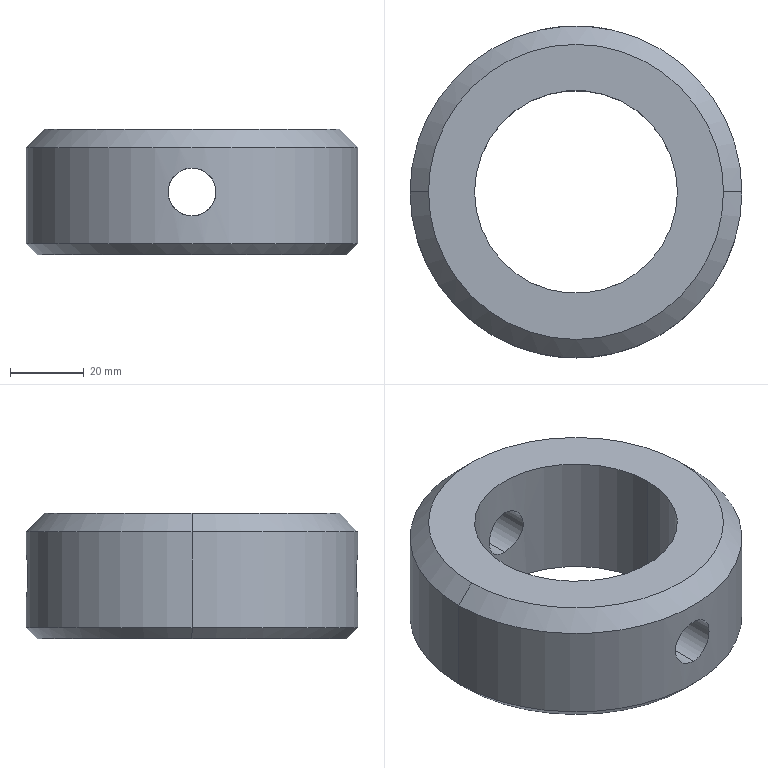Part | SolidWorks | features Chamfer 2, Extrusion 1, ICE 1 | 1 solid | 14 faces | box 90 x 90 x 34 mm | volume 126206 mm3 | cylinder 8 | cone 4 | plane 2 | commonest cylinder face diameters 13 x4 55 x2 90 x2
STEP:
#1=CARTESIAN_POINT('',(-42.,0.,0.));
#2=VERTEX_POINT('',#1);
#3=CARTESIAN_POINT('',(42.,0.,0.));
#4=VERTEX_POINT('',#3);
#5=CARTESIAN_POINT('',(0.,0.,0.));
#6=DIRECTION('',(0.,0.,-1.));
#7=DIRECTION('',(1.,0.,0.));
#8=AXIS2_PLACEMENT_3D('',#5,#6,#7);
#9=CIRCLE('',#8,42.);
#10=EDGE_CURVE('',#2,#4,#9,.T.);
#11=ORIENTED_EDGE('',*,*,#10,.F.);
#12=CARTESIAN_POINT('',(-45.,0.,3.));
#13=VERTEX_POINT('',#12);
#14=CARTESIAN_POINT('',(-45.,0.,3.));
#15=DIRECTION('',(-0.7071,0.,0.7071));
#16=VECTOR('',#15,1000.);
#17=LINE('',#14,#16);
#18=EDGE_CURVE('',#2,#13,#17,.T.);
#19=ORIENTED_EDGE('',*,*,#18,.T.);
#20=CARTESIAN_POINT('',(45.,0.,3.));
#21=VERTEX_POINT('',#20);
#22=CARTESIAN_POINT('',(0.,0.,3.));
#23=DIRECTION('',(0.,0.,1.));
#24=DIRECTION('',(1.,0.,0.));
#25=AXIS2_PLACEMENT_3D('',#22,#23,#24);
#26=CIRCLE('',#25,45.);
#27=EDGE_CURVE('',#21,#13,#26,.T.);
#28=ORIENTED_EDGE('',*,*,#27,.F.);
#29=CARTESIAN_POINT('',(45.,0.,3.));
#30=DIRECTION('',(0.7071,0.,0.7071));
#31=VECTOR('',#30,1000.);
#32=LINE('',#29,#31);
#33=EDGE_CURVE('',#4,#21,#32,.T.);
#34=ORIENTED_EDGE('',*,*,#33,.F.);
#35=EDGE_LOOP('',(#11,#19,#28,#34));
#36=FACE_OUTER_BOUND('',#35,.T.);
#37=CARTESIAN_POINT('',(0.,0.,3.));
#38=DIRECTION('',(0.,0.,1.));
#39=DIRECTION('',(1.,0.,0.));
#40=AXIS2_PLACEMENT_3D('',#37,#38,#39);
#41=CONICAL_SURFACE('',#40,45.,0.7854);
#42=ADVANCED_FACE('',(#36),#41,.T.);
#43=CARTESIAN_POINT('',(40.,0.,34.));
#44=VERTEX_POINT('',#43);
#45=CARTESIAN_POINT('',(-40.,0.,34.));
#46=VERTEX_POINT('',#45);
#47=CARTESIAN_POINT('',(0.,0.,34.));
#48=DIRECTION('',(0.,0.,1.));
#49=DIRECTION('',(1.,0.,0.));
#50=AXIS2_PLACEMENT_3D('',#47,#48,#49);
#51=CIRCLE('',#50,40.);
#52=EDGE_CURVE('',#44,#46,#51,.T.);
#53=ORIENTED_EDGE('',*,*,#52,.F.);
#54=CARTESIAN_POINT('',(45.,0.,29.));
#55=VERTEX_POINT('',#54);
#56=CARTESIAN_POINT('',(40.,0.,34.));
#57=DIRECTION('',(0.7071,0.,-0.7071));
#58=VECTOR('',#57,1000.);
#59=LINE('',#56,#58);
#60=EDGE_CURVE('',#44,#55,#59,.T.);
#61=ORIENTED_EDGE('',*,*,#60,.T.);
#62=CARTESIAN_POINT('',(-45.,0.,29.));
#63=VERTEX_POINT('',#62);
#64=CARTESIAN_POINT('',(0.,0.,29.));
#65=DIRECTION('',(0.,0.,-1.));
#66=DIRECTION('',(1.,0.,0.));
#67=AXIS2_PLACEMENT_3D('',#64,#65,#66);
#68=CIRCLE('',#67,45.);
#69=EDGE_CURVE('',#63,#55,#68,.T.);
#70=ORIENTED_EDGE('',*,*,#69,.F.);
#71=CARTESIAN_POINT('',(-40.,0.,34.));
#72=DIRECTION('',(-0.7071,0.,-0.7071));
#73=VECTOR('',#72,1000.);
#74=LINE('',#71,#73);
#75=EDGE_CURVE('',#46,#63,#74,.T.);
#76=ORIENTED_EDGE('',*,*,#75,.F.);
#77=EDGE_LOOP('',(#53,#61,#70,#76));
#78=FACE_OUTER_BOUND('',#77,.T.);
#79=CARTESIAN_POINT('',(0.,0.,34.));
#80=DIRECTION('',(0.,0.,-1.));
#81=DIRECTION('',(-1.,0.,0.));
#82=AXIS2_PLACEMENT_3D('',#79,#80,#81);
#83=CONICAL_SURFACE('',#82,40.,0.7854);
#84=ADVANCED_FACE('',(#78),#83,.T.);
#85=CARTESIAN_POINT('',(0.,-45.,10.5));
#86=VERTEX_POINT('',#85);
#87=CARTESIAN_POINT('',(0.,-45.,23.5));
#88=VERTEX_POINT('',#87);
#89=CARTESIAN_POINT('',(0.,-45.,10.5));
#90=CARTESIAN_POINT('',(-0.4244,-45.,10.5));
#91=CARTESIAN_POINT('',(-0.8466,-44.994,10.541));
#92=CARTESIAN_POINT('',(-1.477,-44.976,10.666));
#93=CARTESIAN_POINT('',(-1.685,-44.969,10.719));
#94=CARTESIAN_POINT('',(-2.092,-44.952,10.842));
#95=CARTESIAN_POINT('',(-2.491,-44.932,10.985));
#96=CARTESIAN_POINT('',(-2.875,-44.908,11.166));
#97=CARTESIAN_POINT('',(-3.25,-44.883,11.367));
#98=CARTESIAN_POINT('',(-3.434,-44.869,11.477));
#99=CARTESIAN_POINT('',(-3.967,-44.826,11.833));
#100=CARTESIAN_POINT('',(-4.293,-44.796,12.101));
#101=CARTESIAN_POINT('',(-4.893,-44.734,12.7));
#102=CARTESIAN_POINT('',(-5.167,-44.703,13.034));
#103=CARTESIAN_POINT('',(-5.639,-44.646,13.739));
#104=CARTESIAN_POINT('',(-5.839,-44.62,14.112));
#105=CARTESIAN_POINT('',(-6.084,-44.587,14.702));
#106=CARTESIAN_POINT('',(-6.157,-44.577,14.905));
#107=CARTESIAN_POINT('',(-6.281,-44.56,15.313));
#108=CARTESIAN_POINT('',(-6.333,-44.552,15.519));
#109=CARTESIAN_POINT('',(-6.457,-44.534,16.143));
#110=CARTESIAN_POINT('',(-6.5,-44.528,16.566));
#111=CARTESIAN_POINT('',(-6.5,-44.528,17.425));
#112=CARTESIAN_POINT('',(-6.458,-44.534,17.848));
#113=CARTESIAN_POINT('',(-6.335,-44.552,18.472));
#114=CARTESIAN_POINT('',(-6.283,-44.559,18.678));
#115=CARTESIAN_POINT('',(-6.16,-44.576,19.087));
#116=CARTESIAN_POINT('',(-6.087,-44.586,19.29));
#117=CARTESIAN_POINT('',(-5.843,-44.619,19.88));
#118=CARTESIAN_POINT('',(-5.643,-44.645,20.253));
#119=CARTESIAN_POINT('',(-5.172,-44.702,20.96));
#120=CARTESIAN_POINT('',(-4.898,-44.734,21.294));
#121=CARTESIAN_POINT('',(-4.3,-44.795,21.893));
#122=CARTESIAN_POINT('',(-3.974,-44.826,22.162));
#123=CARTESIAN_POINT('',(-3.263,-44.883,22.638));
#124=CARTESIAN_POINT('',(-2.887,-44.909,22.839));
#125=CARTESIAN_POINT('',(-2.3,-44.942,23.083));
#126=CARTESIAN_POINT('',(-2.101,-44.951,23.155));
#127=CARTESIAN_POINT('',(-1.694,-44.969,23.279));
#128=CARTESIAN_POINT('',(-1.485,-44.976,23.332));
#129=CARTESIAN_POINT('',(-0.8549,-44.994,23.458));
#130=CARTESIAN_POINT('',(-0.43,-45.,23.5));
#131=CARTESIAN_POINT('',(0.,-45.,23.5));
#132=B_SPLINE_CURVE_WITH_KNOTS('',3,(#89,#90,#91,#92,#93,#94,#95,#96,#97,#98,#99,#100,#101,#102,#103,#104,#105,#106,#107,#108,#109,#110,#111,#112,#113,#114,#115,#116,#117,#118,#119,#120,#121,#122,#123,#124,#125,#126,#127,#128,#129,#130,#131),.UNSPECIFIED.,.F.,.F.,(4,2,2,1,2,2,2,2,2,2,2,2,2,2,2,2,2,2,2,2,2,4),(0.02035,0.02162,0.02226,0.02289,0.02353,0.02416,0.02543,0.02671,0.02798,0.02861,0.02925,0.03052,0.03179,0.03243,0.03306,0.03433,0.03561,0.03688,0.03815,0.03878,0.03942,0.04069),.UNSPECIFIED.);
#133=EDGE_CURVE('',#86,#88,#132,.T.);
#134=ORIENTED_EDGE('',*,*,#133,.F.);
#135=CARTESIAN_POINT('',(0.,-27.5,10.5));
#136=VERTEX_POINT('',#135);
#137=CARTESIAN_POINT('',(0.,-45.,10.5));
#138=DIRECTION('',(0.,1.,0.));
#139=VECTOR('',#138,1000.);
#140=LINE('',#137,#139);
#141=EDGE_CURVE('',#86,#136,#140,.T.);
#142=ORIENTED_EDGE('',*,*,#141,.T.);
#143=CARTESIAN_POINT('',(0.,-27.5,23.5));
#144=VERTEX_POINT('',#143);
#145=CARTESIAN_POINT('',(0.,-27.5,10.5));
#146=CARTESIAN_POINT('',(-0.425,-27.5,10.5));
#147=CARTESIAN_POINT('',(-0.8485,-27.49,10.541));
#148=CARTESIAN_POINT('',(-1.692,-27.451,10.709));
#149=CARTESIAN_POINT('',(-2.099,-27.423,10.834));
#150=CARTESIAN_POINT('',(-2.687,-27.369,11.077));
#151=CARTESIAN_POINT('',(-2.878,-27.35,11.168));
#152=CARTESIAN_POINT('',(-3.254,-27.307,11.369));
#153=CARTESIAN_POINT('',(-3.439,-27.285,11.48));
#154=CARTESIAN_POINT('',(-3.968,-27.215,11.834));
#155=CARTESIAN_POINT('',(-4.294,-27.164,12.102));
#156=CARTESIAN_POINT('',(-4.894,-27.063,12.701));
#157=CARTESIAN_POINT('',(-5.167,-27.011,13.034));
#158=CARTESIAN_POINT('',(-5.637,-26.917,13.736));
#159=CARTESIAN_POINT('',(-5.837,-26.874,14.109));
#160=CARTESIAN_POINT('',(-6.084,-26.819,14.702));
#161=CARTESIAN_POINT('',(-6.156,-26.802,14.904));
#162=CARTESIAN_POINT('',(-6.28,-26.773,15.311));
#163=CARTESIAN_POINT('',(-6.384,-26.749,15.722));
#164=CARTESIAN_POINT('',(-6.447,-26.734,16.143));
#165=CARTESIAN_POINT('',(-6.489,-26.723,16.567));
#166=CARTESIAN_POINT('',(-6.5,-26.721,16.783));
#167=CARTESIAN_POINT('',(-6.5,-26.721,17.426));
#168=CARTESIAN_POINT('',(-6.458,-26.731,17.849));
#169=CARTESIAN_POINT('',(-6.293,-26.771,18.684));
#170=CARTESIAN_POINT('',(-6.167,-26.8,19.098));
#171=CARTESIAN_POINT('',(-5.841,-26.873,19.883));
#172=CARTESIAN_POINT('',(-5.642,-26.916,20.256));
#173=CARTESIAN_POINT('',(-5.287,-26.987,20.787));
#174=CARTESIAN_POINT('',(-5.159,-27.012,20.96));
#175=CARTESIAN_POINT('',(-4.89,-27.062,21.288));
#176=CARTESIAN_POINT('',(-4.748,-27.087,21.444));
#177=CARTESIAN_POINT('',(-4.301,-27.163,21.892));
#178=CARTESIAN_POINT('',(-3.972,-27.214,22.163));
#179=CARTESIAN_POINT('',(-3.263,-27.308,22.638));
#180=CARTESIAN_POINT('',(-2.89,-27.351,22.838));
#181=CARTESIAN_POINT('',(-2.303,-27.404,23.082));
#182=CARTESIAN_POINT('',(-2.103,-27.42,23.154));
#183=CARTESIAN_POINT('',(-1.693,-27.449,23.279));
#184=CARTESIAN_POINT('',(-1.484,-27.461,23.332));
#185=CARTESIAN_POINT('',(-0.8559,-27.49,23.458));
#186=CARTESIAN_POINT('',(-0.431,-27.5,23.5));
#187=CARTESIAN_POINT('',(0.,-27.5,23.5));
#188=B_SPLINE_CURVE_WITH_KNOTS('',3,(#145,#146,#147,#148,#149,#150,#151,#152,#153,#154,#155,#156,#157,#158,#159,#160,#161,#162,#163,#164,#165,#166,#167,#168,#169,#170,#171,#172,#173,#174,#175,#176,#177,#178,#179,#180,#181,#182,#183,#184,#185,#186,#187),.UNSPECIFIED.,.F.,.F.,(4,2,2,2,2,2,2,2,2,1,2,2,2,2,2,2,2,2,2,2,2,4),(0.02039,0.02167,0.02294,0.02358,0.02422,0.02549,0.02677,0.02804,0.02868,0.02931,0.02995,0.03059,0.03186,0.03314,0.03441,0.03505,0.03569,0.03696,0.03823,0.03887,0.03951,0.04078),.UNSPECIFIED.);
#189=EDGE_CURVE('',#136,#144,#188,.T.);
#190=ORIENTED_EDGE('',*,*,#189,.T.);
#191=CARTESIAN_POINT('',(0.,-45.,23.5));
#192=DIRECTION('',(0.,1.,0.));
#193=VECTOR('',#192,1000.);
#194=LINE('',#191,#193);
#195=EDGE_CURVE('',#88,#144,#194,.T.);
#196=ORIENTED_EDGE('',*,*,#195,.F.);
#197=EDGE_LOOP('',(#134,#142,#190,#196));
#198=FACE_OUTER_BOUND('',#197,.T.);
#199=CARTESIAN_POINT('',(0.,-45.,17.));
#200=DIRECTION('',(0.,1.,0.));
#201=DIRECTION('',(0.,0.,1.));
#202=AXIS2_PLACEMENT_3D('',#199,#200,#201);
#203=CYLINDRICAL_SURFACE('',#202,6.5);
#204=ADVANCED_FACE('',(#198),#203,.F.);
#205=CARTESIAN_POINT('',(0.,27.5,23.5));
#206=VERTEX_POINT('',#205);
#207=CARTESIAN_POINT('',(0.,27.5,10.5));
#208=VERTEX_POINT('',#207);
#209=CARTESIAN_POINT('',(0.,27.5,23.5));
#210=CARTESIAN_POINT('',(-0.4311,27.5,23.5));
#211=CARTESIAN_POINT('',(-0.8547,27.49,23.458));
#212=CARTESIAN_POINT('',(-1.479,27.461,23.333));
#213=CARTESIAN_POINT('',(-1.686,27.449,23.281));
#214=CARTESIAN_POINT('',(-2.095,27.421,23.157));
#215=CARTESIAN_POINT('',(-2.298,27.405,23.084));
#216=CARTESIAN_POINT('',(-2.888,27.351,22.839));
#217=CARTESIAN_POINT('',(-3.261,27.308,22.639));
#218=CARTESIAN_POINT('',(-3.79,27.238,22.285));
#219=CARTESIAN_POINT('',(-3.962,27.214,22.157));
#220=CARTESIAN_POINT('',(-4.291,27.164,21.887));
#221=CARTESIAN_POINT('',(-4.448,27.138,21.744));
#222=CARTESIAN_POINT('',(-4.896,27.062,21.296));
#223=CARTESIAN_POINT('',(-5.165,27.012,20.97));
#224=CARTESIAN_POINT('',(-5.64,26.917,20.26));
#225=CARTESIAN_POINT('',(-5.841,26.873,19.884));
#226=CARTESIAN_POINT('',(-6.084,26.819,19.298));
#227=CARTESIAN_POINT('',(-6.156,26.802,19.098));
#228=CARTESIAN_POINT('',(-6.28,26.773,18.69));
#229=CARTESIAN_POINT('',(-6.333,26.761,18.481));
#230=CARTESIAN_POINT('',(-6.458,26.731,17.851));
#231=CARTESIAN_POINT('',(-6.5,26.721,17.428));
#232=CARTESIAN_POINT('',(-6.5,26.721,16.577));
#233=CARTESIAN_POINT('',(-6.458,26.731,16.145));
#234=CARTESIAN_POINT('',(-6.291,26.771,15.31));
#235=CARTESIAN_POINT('',(-6.167,26.8,14.904));
#236=CARTESIAN_POINT('',(-5.922,26.855,14.312));
#237=CARTESIAN_POINT('',(-5.83,26.875,14.117));
#238=CARTESIAN_POINT('',(-5.629,26.918,13.743));
#239=CARTESIAN_POINT('',(-5.52,26.941,13.561));
#240=CARTESIAN_POINT('',(-5.285,26.988,13.21));
#241=CARTESIAN_POINT('',(-5.159,27.012,13.04));
#242=CARTESIAN_POINT('',(-4.89,27.062,12.712));
#243=CARTESIAN_POINT('',(-4.746,27.088,12.554));
#244=CARTESIAN_POINT('',(-4.294,27.164,12.102));
#245=CARTESIAN_POINT('',(-3.967,27.215,11.834));
#246=CARTESIAN_POINT('',(-3.265,27.308,11.363));
#247=CARTESIAN_POINT('',(-2.884,27.351,11.159));
#248=CARTESIAN_POINT('',(-2.099,27.423,10.833));
#249=CARTESIAN_POINT('',(-1.693,27.451,10.71));
#250=CARTESIAN_POINT('',(-1.066,27.48,10.584));
#251=CARTESIAN_POINT('',(-0.8521,27.488,10.553));
#252=CARTESIAN_POINT('',(-0.4255,27.498,10.51));
#253=CARTESIAN_POINT('',(-0.2125,27.5,10.5));
#254=CARTESIAN_POINT('',(0.,27.5,10.5));
#255=B_SPLINE_CURVE_WITH_KNOTS('',3,(#209,#210,#211,#212,#213,#214,#215,#216,#217,#218,#219,#220,#221,#222,#223,#224,#225,#226,#227,#228,#229,#230,#231,#232,#233,#234,#235,#236,#237,#238,#239,#240,#241,#242,#243,#244,#245,#246,#247,#248,#249,#250,#251,#252,#253,#254),.UNSPECIFIED.,.F.,.F.,(4,2,2,2,2,2,2,2,2,2,2,2,2,2,2,2,2,2,2,2,2,2,4),(0.,0.001275,0.001912,0.002549,0.003824,0.004461,0.005099,0.006373,0.007648,0.008285,0.008923,0.0102,0.01147,0.01275,0.01338,0.01402,0.01466,0.0153,0.01657,0.01785,0.01912,0.01976,0.02039),.UNSPECIFIED.);
#256=EDGE_CURVE('',#206,#208,#255,.T.);
#257=ORIENTED_EDGE('',*,*,#256,.T.);
#258=CARTESIAN_POINT('',(0.,45.,10.5));
#259=VERTEX_POINT('',#258);
#260=CARTESIAN_POINT('',(0.,-45.,10.5));
#261=DIRECTION('',(0.,1.,0.));
#262=VECTOR('',#261,1000.);
#263=LINE('',#260,#262);
#264=EDGE_CURVE('',#208,#259,#263,.T.);
#265=ORIENTED_EDGE('',*,*,#264,.T.);
#266=CARTESIAN_POINT('',(0.,45.,23.5));
#267=VERTEX_POINT('',#266);
#268=CARTESIAN_POINT('',(0.,45.,23.5));
#269=CARTESIAN_POINT('',(-0.4301,45.,23.5));
#270=CARTESIAN_POINT('',(-0.8529,44.994,23.458));
#271=CARTESIAN_POINT('',(-1.477,44.976,23.334));
#272=CARTESIAN_POINT('',(-1.683,44.969,23.282));
#273=CARTESIAN_POINT('',(-2.091,44.952,23.158));
#274=CARTESIAN_POINT('',(-2.294,44.942,23.085));
#275=CARTESIAN_POINT('',(-2.885,44.909,22.84));
#276=CARTESIAN_POINT('',(-3.258,44.883,22.641));
#277=CARTESIAN_POINT('',(-3.964,44.826,22.169));
#278=CARTESIAN_POINT('',(-4.298,44.795,21.895));
#279=CARTESIAN_POINT('',(-4.897,44.734,21.296));
#280=CARTESIAN_POINT('',(-5.165,44.703,20.969));
#281=CARTESIAN_POINT('',(-5.522,44.66,20.436));
#282=CARTESIAN_POINT('',(-5.632,44.646,20.252));
#283=CARTESIAN_POINT('',(-5.833,44.621,19.877));
#284=CARTESIAN_POINT('',(-6.014,44.597,19.494));
#285=CARTESIAN_POINT('',(-6.157,44.577,19.095));
#286=CARTESIAN_POINT('',(-6.281,44.56,18.688));
#287=CARTESIAN_POINT('',(-6.333,44.552,18.479));
#288=CARTESIAN_POINT('',(-6.458,44.534,17.849));
#289=CARTESIAN_POINT('',(-6.5,44.528,17.427));
#290=CARTESIAN_POINT('',(-6.5,44.528,16.578));
#291=CARTESIAN_POINT('',(-6.458,44.534,16.147));
#292=CARTESIAN_POINT('',(-6.291,44.558,15.312));
#293=CARTESIAN_POINT('',(-6.169,44.576,14.907));
#294=CARTESIAN_POINT('',(-5.924,44.608,14.316));
#295=CARTESIAN_POINT('',(-5.832,44.621,14.121));
#296=CARTESIAN_POINT('',(-5.631,44.646,13.745));
#297=CARTESIAN_POINT('',(-5.521,44.66,13.564));
#298=CARTESIAN_POINT('',(-5.169,44.703,13.036));
#299=CARTESIAN_POINT('',(-4.899,44.734,12.707));
#300=CARTESIAN_POINT('',(-4.294,44.796,12.101));
#301=CARTESIAN_POINT('',(-3.966,44.826,11.833));
#302=CARTESIAN_POINT('',(-3.438,44.869,11.48));
#303=CARTESIAN_POINT('',(-3.256,44.882,11.37));
#304=CARTESIAN_POINT('',(-2.88,44.908,11.169));
#305=CARTESIAN_POINT('',(-2.685,44.92,11.077));
#306=CARTESIAN_POINT('',(-2.095,44.953,10.832));
#307=CARTESIAN_POINT('',(-1.69,44.97,10.709));
#308=CARTESIAN_POINT('',(-0.8557,44.994,10.543));
#309=CARTESIAN_POINT('',(-0.4245,45.,10.5));
#310=CARTESIAN_POINT('',(0.,45.,10.5));
#311=B_SPLINE_CURVE_WITH_KNOTS('',3,(#268,#269,#270,#271,#272,#273,#274,#275,#276,#277,#278,#279,#280,#281,#282,#283,#284,#285,#286,#287,#288,#289,#290,#291,#292,#293,#294,#295,#296,#297,#298,#299,#300,#301,#302,#303,#304,#305,#306,#307,#308,#309,#310),.UNSPECIFIED.,.F.,.F.,(4,2,2,2,2,2,2,2,1,2,2,2,2,2,2,2,2,2,2,2,2,4),(0.,0.001272,0.001908,0.002544,0.003815,0.005087,0.006359,0.006995,0.007631,0.008267,0.008903,0.01017,0.01145,0.01272,0.01335,0.01399,0.01526,0.01653,0.01717,0.01781,0.01908,0.02035),.UNSPECIFIED.);
#312=EDGE_CURVE('',#267,#259,#311,.T.);
#313=ORIENTED_EDGE('',*,*,#312,.F.);
#314=CARTESIAN_POINT('',(0.,-45.,23.5));
#315=DIRECTION('',(0.,1.,0.));
#316=VECTOR('',#315,1000.);
#317=LINE('',#314,#316);
#318=EDGE_CURVE('',#206,#267,#317,.T.);
#319=ORIENTED_EDGE('',*,*,#318,.F.);
#320=EDGE_LOOP('',(#257,#265,#313,#319));
#321=FACE_OUTER_BOUND('',#320,.T.);
#322=CARTESIAN_POINT('',(0.,-45.,17.));
#323=DIRECTION('',(0.,1.,0.));
#324=DIRECTION('',(0.,0.,1.));
#325=AXIS2_PLACEMENT_3D('',#322,#323,#324);
#326=CYLINDRICAL_SURFACE('',#325,6.5);
#327=ADVANCED_FACE('',(#321),#326,.F.);
#328=CARTESIAN_POINT('',(0.,-27.5,23.5));
#329=CARTESIAN_POINT('',(0.4311,-27.5,23.5));
#330=CARTESIAN_POINT('',(0.8547,-27.49,23.458));
#331=CARTESIAN_POINT('',(1.479,-27.461,23.333));
#332=CARTESIAN_POINT('',(1.686,-27.449,23.281));
#333=CARTESIAN_POINT('',(2.095,-27.421,23.157));
#334=CARTESIAN_POINT('',(2.298,-27.405,23.084));
#335=CARTESIAN_POINT('',(2.888,-27.351,22.839));
#336=CARTESIAN_POINT('',(3.261,-27.308,22.639));
#337=CARTESIAN_POINT('',(3.79,-27.238,22.285));
#338=CARTESIAN_POINT('',(3.962,-27.214,22.157));
#339=CARTESIAN_POINT('',(4.291,-27.164,21.887));
#340=CARTESIAN_POINT('',(4.448,-27.138,21.744));
#341=CARTESIAN_POINT('',(4.896,-27.062,21.296));
#342=CARTESIAN_POINT('',(5.165,-27.012,20.97));
#343=CARTESIAN_POINT('',(5.64,-26.917,20.26));
#344=CARTESIAN_POINT('',(5.841,-26.873,19.884));
#345=CARTESIAN_POINT('',(6.084,-26.819,19.298));
#346=CARTESIAN_POINT('',(6.156,-26.802,19.098));
#347=CARTESIAN_POINT('',(6.28,-26.773,18.69));
#348=CARTESIAN_POINT('',(6.333,-26.761,18.481));
#349=CARTESIAN_POINT('',(6.458,-26.731,17.851));
#350=CARTESIAN_POINT('',(6.5,-26.721,17.428));
#351=CARTESIAN_POINT('',(6.5,-26.721,16.577));
#352=CARTESIAN_POINT('',(6.458,-26.731,16.145));
#353=CARTESIAN_POINT('',(6.291,-26.771,15.31));
#354=CARTESIAN_POINT('',(6.167,-26.8,14.904));
#355=CARTESIAN_POINT('',(5.922,-26.855,14.312));
#356=CARTESIAN_POINT('',(5.83,-26.875,14.117));
#357=CARTESIAN_POINT('',(5.629,-26.918,13.743));
#358=CARTESIAN_POINT('',(5.52,-26.941,13.561));
#359=CARTESIAN_POINT('',(5.285,-26.988,13.21));
#360=CARTESIAN_POINT('',(5.159,-27.012,13.04));
#361=CARTESIAN_POINT('',(4.89,-27.062,12.712));
#362=CARTESIAN_POINT('',(4.746,-27.088,12.554));
#363=CARTESIAN_POINT('',(4.294,-27.164,12.102));
#364=CARTESIAN_POINT('',(3.967,-27.215,11.834));
#365=CARTESIAN_POINT('',(3.265,-27.308,11.363));
#366=CARTESIAN_POINT('',(2.884,-27.351,11.159));
#367=CARTESIAN_POINT('',(2.099,-27.423,10.833));
#368=CARTESIAN_POINT('',(1.693,-27.451,10.71));
#369=CARTESIAN_POINT('',(1.066,-27.48,10.584));
#370=CARTESIAN_POINT('',(0.8521,-27.488,10.553));
#371=CARTESIAN_POINT('',(0.4255,-27.498,10.51));
#372=CARTESIAN_POINT('',(0.2125,-27.5,10.5));
#373=CARTESIAN_POINT('',(0.,-27.5,10.5));
#374=B_SPLINE_CURVE_WITH_KNOTS('',3,(#328,#329,#330,#331,#332,#333,#334,#335,#336,#337,#338,#339,#340,#341,#342,#343,#344,#345,#346,#347,#348,#349,#350,#351,#352,#353,#354,#355,#356,#357,#358,#359,#360,#361,#362,#363,#364,#365,#366,#367,#368,#369,#370,#371,#372,#373),.UNSPECIFIED.,.F.,.F.,(4,2,2,2,2,2,2,2,2,2,2,2,2,2,2,2,2,2,2,2,2,2,4),(0.,0.001275,0.001912,0.002549,0.003824,0.004461,0.005099,0.006373,0.007648,0.008285,0.008923,0.0102,0.01147,0.01275,0.01338,0.01402,0.01466,0.0153,0.01657,0.01785,0.01912,0.01976,0.02039),.UNSPECIFIED.);
#375=EDGE_CURVE('',#144,#136,#374,.T.);
#376=ORIENTED_EDGE('',*,*,#375,.F.);
#377=ORIENTED_EDGE('',*,*,#189,.F.);
#378=EDGE_LOOP('',(#376,#377));
#379=FACE_BOUND('',#378,.T.);
#380=CARTESIAN_POINT('',(-27.5,0.,34.));
#381=VERTEX_POINT('',#380);
#382=CARTESIAN_POINT('',(27.5,0.,34.));
#383=VERTEX_POINT('',#382);
#384=CARTESIAN_POINT('',(0.,0.,34.));
#385=DIRECTION('',(0.,0.,1.));
#386=DIRECTION('',(1.,0.,0.));
#387=AXIS2_PLACEMENT_3D('',#384,#385,#386);
#388=CIRCLE('',#387,27.5);
#389=EDGE_CURVE('',#381,#383,#388,.T.);
#390=ORIENTED_EDGE('',*,*,#389,.T.);
#391=CARTESIAN_POINT('',(27.5,0.,0.));
#392=VERTEX_POINT('',#391);
#393=CARTESIAN_POINT('',(27.5,0.,34.));
#394=DIRECTION('',(0.,0.,-1.));
#395=VECTOR('',#394,1000.);
#396=LINE('',#393,#395);
#397=EDGE_CURVE('',#383,#392,#396,.T.);
#398=ORIENTED_EDGE('',*,*,#397,.T.);
#399=CARTESIAN_POINT('',(-27.5,0.,0.));
#400=VERTEX_POINT('',#399);
#401=CARTESIAN_POINT('',(0.,0.,0.));
#402=DIRECTION('',(0.,0.,1.));
#403=DIRECTION('',(1.,0.,0.));
#404=AXIS2_PLACEMENT_3D('',#401,#402,#403);
#405=CIRCLE('',#404,27.5);
#406=EDGE_CURVE('',#400,#392,#405,.T.);
#407=ORIENTED_EDGE('',*,*,#406,.F.);
#408=CARTESIAN_POINT('',(-27.5,0.,34.));
#409=DIRECTION('',(0.,0.,-1.));
#410=VECTOR('',#409,1000.);
#411=LINE('',#408,#410);
#412=EDGE_CURVE('',#381,#400,#411,.T.);
#413=ORIENTED_EDGE('',*,*,#412,.F.);
#414=EDGE_LOOP('',(#390,#398,#407,#413));
#415=FACE_OUTER_BOUND('',#414,.T.);
#416=CARTESIAN_POINT('',(0.,0.,34.));
#417=DIRECTION('',(0.,0.,-1.));
#418=DIRECTION('',(-1.,0.,0.));
#419=AXIS2_PLACEMENT_3D('',#416,#417,#418);
#420=CYLINDRICAL_SURFACE('',#419,27.5);
#421=ADVANCED_FACE('',(#379,#415),#420,.F.);
#422=ORIENTED_EDGE('',*,*,#312,.T.);
#423=CARTESIAN_POINT('',(0.,45.,10.5));
#424=CARTESIAN_POINT('',(0.4244,45.,10.5));
#425=CARTESIAN_POINT('',(0.8466,44.994,10.541));
#426=CARTESIAN_POINT('',(1.477,44.976,10.666));
#427=CARTESIAN_POINT('',(1.685,44.969,10.719));
#428=CARTESIAN_POINT('',(2.092,44.952,10.842));
#429=CARTESIAN_POINT('',(2.491,44.932,10.985));
#430=CARTESIAN_POINT('',(2.875,44.908,11.166));
#431=CARTESIAN_POINT('',(3.25,44.883,11.367));
#432=CARTESIAN_POINT('',(3.434,44.869,11.477));
#433=CARTESIAN_POINT('',(3.967,44.826,11.833));
#434=CARTESIAN_POINT('',(4.293,44.796,12.101));
#435=CARTESIAN_POINT('',(4.893,44.734,12.7));
#436=CARTESIAN_POINT('',(5.167,44.703,13.034));
#437=CARTESIAN_POINT('',(5.639,44.646,13.739));
#438=CARTESIAN_POINT('',(5.839,44.62,14.112));
#439=CARTESIAN_POINT('',(6.084,44.587,14.702));
#440=CARTESIAN_POINT('',(6.157,44.577,14.905));
#441=CARTESIAN_POINT('',(6.281,44.56,15.313));
#442=CARTESIAN_POINT('',(6.333,44.552,15.519));
#443=CARTESIAN_POINT('',(6.457,44.534,16.143));
#444=CARTESIAN_POINT('',(6.5,44.528,16.566));
#445=CARTESIAN_POINT('',(6.5,44.528,17.425));
#446=CARTESIAN_POINT('',(6.458,44.534,17.848));
#447=CARTESIAN_POINT('',(6.335,44.552,18.472));
#448=CARTESIAN_POINT('',(6.283,44.559,18.678));
#449=CARTESIAN_POINT('',(6.16,44.576,19.087));
#450=CARTESIAN_POINT('',(6.087,44.586,19.29));
#451=CARTESIAN_POINT('',(5.843,44.619,19.88));
#452=CARTESIAN_POINT('',(5.643,44.645,20.253));
#453=CARTESIAN_POINT('',(5.172,44.702,20.96));
#454=CARTESIAN_POINT('',(4.898,44.734,21.294));
#455=CARTESIAN_POINT('',(4.3,44.795,21.893));
#456=CARTESIAN_POINT('',(3.974,44.826,22.162));
#457=CARTESIAN_POINT('',(3.263,44.883,22.638));
#458=CARTESIAN_POINT('',(2.887,44.909,22.839));
#459=CARTESIAN_POINT('',(2.3,44.942,23.083));
#460=CARTESIAN_POINT('',(2.101,44.951,23.155));
#461=CARTESIAN_POINT('',(1.694,44.969,23.279));
#462=CARTESIAN_POINT('',(1.485,44.976,23.332));
#463=CARTESIAN_POINT('',(0.8549,44.994,23.458));
#464=CARTESIAN_POINT('',(0.43,45.,23.5));
#465=CARTESIAN_POINT('',(0.,45.,23.5));
#466=B_SPLINE_CURVE_WITH_KNOTS('',3,(#423,#424,#425,#426,#427,#428,#429,#430,#431,#432,#433,#434,#435,#436,#437,#438,#439,#440,#441,#442,#443,#444,#445,#446,#447,#448,#449,#450,#451,#452,#453,#454,#455,#456,#457,#458,#459,#460,#461,#462,#463,#464,#465),.UNSPECIFIED.,.F.,.F.,(4,2,2,1,2,2,2,2,2,2,2,2,2,2,2,2,2,2,2,2,2,4),(0.02035,0.02162,0.02226,0.02289,0.02353,0.02416,0.02543,0.02671,0.02798,0.02861,0.02925,0.03052,0.03179,0.03243,0.03306,0.03433,0.03561,0.03688,0.03815,0.03878,0.03942,0.04069),.UNSPECIFIED.);
#467=EDGE_CURVE('',#259,#267,#466,.T.);
#468=ORIENTED_EDGE('',*,*,#467,.T.);
#469=EDGE_LOOP('',(#422,#468));
#470=FACE_BOUND('',#469,.T.);
#471=ORIENTED_EDGE('',*,*,#69,.T.);
#472=CARTESIAN_POINT('',(45.,0.,34.));
#473=DIRECTION('',(0.,0.,-1.));
#474=VECTOR('',#473,1000.);
#475=LINE('',#472,#474);
#476=EDGE_CURVE('',#55,#21,#475,.T.);
#477=ORIENTED_EDGE('',*,*,#476,.T.);
#478=ORIENTED_EDGE('',*,*,#27,.T.);
#479=CARTESIAN_POINT('',(-45.,0.,34.));
#480=DIRECTION('',(0.,0.,-1.));
#481=VECTOR('',#480,1000.);
#482=LINE('',#479,#481);
#483=EDGE_CURVE('',#63,#13,#482,.T.);
#484=ORIENTED_EDGE('',*,*,#483,.F.);
#485=EDGE_LOOP('',(#471,#477,#478,#484));
#486=FACE_OUTER_BOUND('',#485,.T.);
#487=CARTESIAN_POINT('',(0.,0.,34.));
#488=DIRECTION('',(0.,0.,-1.));
#489=DIRECTION('',(-1.,0.,0.));
#490=AXIS2_PLACEMENT_3D('',#487,#488,#489);
#491=CYLINDRICAL_SURFACE('',#490,45.);
#492=ADVANCED_FACE('',(#470,#486),#491,.T.);
#493=CARTESIAN_POINT('',(0.,0.,34.));
#494=DIRECTION('',(0.,0.,1.));
#495=DIRECTION('',(1.,0.,0.));
#496=AXIS2_PLACEMENT_3D('',#493,#494,#495);
#497=CIRCLE('',#496,40.);
#498=EDGE_CURVE('',#46,#44,#497,.T.);
#499=ORIENTED_EDGE('',*,*,#498,.T.);
#500=ORIENTED_EDGE('',*,*,#52,.T.);
#501=EDGE_LOOP('',(#499,#500));
#502=FACE_OUTER_BOUND('',#501,.T.);
#503=ORIENTED_EDGE('',*,*,#389,.F.);
#504=CARTESIAN_POINT('',(0.,0.,34.));
#505=DIRECTION('',(0.,0.,1.));
#506=DIRECTION('',(1.,0.,0.));
#507=AXIS2_PLACEMENT_3D('',#504,#505,#506);
#508=CIRCLE('',#507,27.5);
#509=EDGE_CURVE('',#383,#381,#508,.T.);
#510=ORIENTED_EDGE('',*,*,#509,.F.);
#511=EDGE_LOOP('',(#503,#510));
#512=FACE_BOUND('',#511,.T.);
#513=CARTESIAN_POINT('',(0.,0.,34.));
#514=DIRECTION('',(0.,0.,1.));
#515=DIRECTION('',(1.,0.,0.));
#516=AXIS2_PLACEMENT_3D('',#513,#514,#515);
#517=PLANE('',#516);
#518=ADVANCED_FACE('',(#502,#512),#517,.T.);
#519=CARTESIAN_POINT('',(0.,0.,0.));
#520=DIRECTION('',(0.,0.,-1.));
#521=DIRECTION('',(1.,0.,0.));
#522=AXIS2_PLACEMENT_3D('',#519,#520,#521);
#523=CIRCLE('',#522,42.);
#524=EDGE_CURVE('',#4,#2,#523,.T.);
#525=ORIENTED_EDGE('',*,*,#524,.T.);
#526=ORIENTED_EDGE('',*,*,#10,.T.);
#527=EDGE_LOOP('',(#525,#526));
#528=FACE_OUTER_BOUND('',#527,.T.);
#529=ORIENTED_EDGE('',*,*,#406,.T.);
#530=CARTESIAN_POINT('',(0.,0.,0.));
#531=DIRECTION('',(0.,0.,1.));
#532=DIRECTION('',(1.,0.,0.));
#533=AXIS2_PLACEMENT_3D('',#530,#531,#532);
#534=CIRCLE('',#533,27.5);
#535=EDGE_CURVE('',#392,#400,#534,.T.);
#536=ORIENTED_EDGE('',*,*,#535,.T.);
#537=EDGE_LOOP('',(#529,#536));
#538=FACE_BOUND('',#537,.T.);
#539=CARTESIAN_POINT('',(0.,0.,0.));
#540=DIRECTION('',(0.,0.,1.));
#541=DIRECTION('',(1.,0.,0.));
#542=AXIS2_PLACEMENT_3D('',#539,#540,#541);
#543=PLANE('',#542);
#544=ADVANCED_FACE('',(#528,#538),#543,.F.);
#545=ORIENTED_EDGE('',*,*,#476,.F.);
#546=CARTESIAN_POINT('',(0.,0.,29.));
#547=DIRECTION('',(0.,0.,-1.));
#548=DIRECTION('',(1.,0.,0.));
#549=AXIS2_PLACEMENT_3D('',#546,#547,#548);
#550=CIRCLE('',#549,45.);
#551=EDGE_CURVE('',#55,#63,#550,.T.);
#552=ORIENTED_EDGE('',*,*,#551,.T.);
#553=ORIENTED_EDGE('',*,*,#483,.T.);
#554=CARTESIAN_POINT('',(0.,0.,3.));
#555=DIRECTION('',(0.,0.,1.));
#556=DIRECTION('',(1.,0.,0.));
#557=AXIS2_PLACEMENT_3D('',#554,#555,#556);
#558=CIRCLE('',#557,45.);
#559=EDGE_CURVE('',#13,#21,#558,.T.);
#560=ORIENTED_EDGE('',*,*,#559,.T.);
#561=EDGE_LOOP('',(#545,#552,#553,#560));
#562=FACE_OUTER_BOUND('',#561,.T.);
#563=CARTESIAN_POINT('',(0.,-45.,23.5));
#564=CARTESIAN_POINT('',(0.4301,-45.,23.5));
#565=CARTESIAN_POINT('',(0.8529,-44.994,23.458));
#566=CARTESIAN_POINT('',(1.477,-44.976,23.334));
#567=CARTESIAN_POINT('',(1.683,-44.969,23.282));
#568=CARTESIAN_POINT('',(2.091,-44.952,23.158));
#569=CARTESIAN_POINT('',(2.294,-44.942,23.085));
#570=CARTESIAN_POINT('',(2.885,-44.909,22.84));
#571=CARTESIAN_POINT('',(3.258,-44.883,22.641));
#572=CARTESIAN_POINT('',(3.964,-44.826,22.169));
#573=CARTESIAN_POINT('',(4.298,-44.795,21.895));
#574=CARTESIAN_POINT('',(4.897,-44.734,21.296));
#575=CARTESIAN_POINT('',(5.165,-44.703,20.969));
#576=CARTESIAN_POINT('',(5.522,-44.66,20.436));
#577=CARTESIAN_POINT('',(5.632,-44.646,20.252));
#578=CARTESIAN_POINT('',(5.833,-44.621,19.877));
#579=CARTESIAN_POINT('',(6.014,-44.597,19.494));
#580=CARTESIAN_POINT('',(6.157,-44.577,19.095));
#581=CARTESIAN_POINT('',(6.281,-44.56,18.688));
#582=CARTESIAN_POINT('',(6.333,-44.552,18.479));
#583=CARTESIAN_POINT('',(6.458,-44.534,17.849));
#584=CARTESIAN_POINT('',(6.5,-44.528,17.427));
#585=CARTESIAN_POINT('',(6.5,-44.528,16.578));
#586=CARTESIAN_POINT('',(6.458,-44.534,16.147));
#587=CARTESIAN_POINT('',(6.291,-44.558,15.312));
#588=CARTESIAN_POINT('',(6.169,-44.576,14.907));
#589=CARTESIAN_POINT('',(5.924,-44.608,14.316));
#590=CARTESIAN_POINT('',(5.832,-44.621,14.121));
#591=CARTESIAN_POINT('',(5.631,-44.646,13.745));
#592=CARTESIAN_POINT('',(5.521,-44.66,13.564));
#593=CARTESIAN_POINT('',(5.169,-44.703,13.036));
#594=CARTESIAN_POINT('',(4.899,-44.734,12.707));
#595=CARTESIAN_POINT('',(4.294,-44.796,12.101));
#596=CARTESIAN_POINT('',(3.966,-44.826,11.833));
#597=CARTESIAN_POINT('',(3.438,-44.869,11.48));
#598=CARTESIAN_POINT('',(3.256,-44.882,11.37));
#599=CARTESIAN_POINT('',(2.88,-44.908,11.169));
#600=CARTESIAN_POINT('',(2.685,-44.92,11.077));
#601=CARTESIAN_POINT('',(2.095,-44.953,10.832));
#602=CARTESIAN_POINT('',(1.69,-44.97,10.709));
#603=CARTESIAN_POINT('',(0.8557,-44.994,10.543));
#604=CARTESIAN_POINT('',(0.4245,-45.,10.5));
#605=CARTESIAN_POINT('',(0.,-45.,10.5));
#606=B_SPLINE_CURVE_WITH_KNOTS('',3,(#563,#564,#565,#566,#567,#568,#569,#570,#571,#572,#573,#574,#575,#576,#577,#578,#579,#580,#581,#582,#583,#584,#585,#586,#587,#588,#589,#590,#591,#592,#593,#594,#595,#596,#597,#598,#599,#600,#601,#602,#603,#604,#605),.UNSPECIFIED.,.F.,.F.,(4,2,2,2,2,2,2,2,1,2,2,2,2,2,2,2,2,2,2,2,2,4),(0.,0.001272,0.001908,0.002544,0.003815,0.005087,0.006359,0.006995,0.007631,0.008267,0.008903,0.01017,0.01145,0.01272,0.01335,0.01399,0.01526,0.01653,0.01717,0.01781,0.01908,0.02035),.UNSPECIFIED.);
#607=EDGE_CURVE('',#88,#86,#606,.T.);
#608=ORIENTED_EDGE('',*,*,#607,.T.);
#609=ORIENTED_EDGE('',*,*,#133,.T.);
#610=EDGE_LOOP('',(#608,#609));
#611=FACE_BOUND('',#610,.T.);
#612=CARTESIAN_POINT('',(0.,0.,34.));
#613=DIRECTION('',(0.,0.,-1.));
#614=DIRECTION('',(-1.,0.,0.));
#615=AXIS2_PLACEMENT_3D('',#612,#613,#614);
#616=CYLINDRICAL_SURFACE('',#615,45.);
#617=ADVANCED_FACE('',(#562,#611),#616,.T.);
#618=ORIENTED_EDGE('',*,*,#397,.F.);
#619=ORIENTED_EDGE('',*,*,#509,.T.);
#620=ORIENTED_EDGE('',*,*,#412,.T.);
#621=ORIENTED_EDGE('',*,*,#535,.F.);
#622=EDGE_LOOP('',(#618,#619,#620,#621));
#623=FACE_OUTER_BOUND('',#622,.T.);
#624=ORIENTED_EDGE('',*,*,#256,.F.);
#625=CARTESIAN_POINT('',(0.,27.5,10.5));
#626=CARTESIAN_POINT('',(0.425,27.5,10.5));
#627=CARTESIAN_POINT('',(0.8485,27.49,10.541));
#628=CARTESIAN_POINT('',(1.692,27.451,10.709));
#629=CARTESIAN_POINT('',(2.099,27.423,10.834));
#630=CARTESIAN_POINT('',(2.687,27.369,11.077));
#631=CARTESIAN_POINT('',(2.878,27.35,11.168));
#632=CARTESIAN_POINT('',(3.254,27.307,11.369));
#633=CARTESIAN_POINT('',(3.439,27.285,11.48));
#634=CARTESIAN_POINT('',(3.968,27.215,11.834));
#635=CARTESIAN_POINT('',(4.294,27.164,12.102));
#636=CARTESIAN_POINT('',(4.894,27.063,12.701));
#637=CARTESIAN_POINT('',(5.167,27.011,13.034));
#638=CARTESIAN_POINT('',(5.637,26.917,13.736));
#639=CARTESIAN_POINT('',(5.837,26.874,14.109));
#640=CARTESIAN_POINT('',(6.084,26.819,14.702));
#641=CARTESIAN_POINT('',(6.156,26.802,14.904));
#642=CARTESIAN_POINT('',(6.28,26.773,15.311));
#643=CARTESIAN_POINT('',(6.384,26.749,15.722));
#644=CARTESIAN_POINT('',(6.447,26.734,16.143));
#645=CARTESIAN_POINT('',(6.489,26.723,16.567));
#646=CARTESIAN_POINT('',(6.5,26.721,16.783));
#647=CARTESIAN_POINT('',(6.5,26.721,17.426));
#648=CARTESIAN_POINT('',(6.458,26.731,17.849));
#649=CARTESIAN_POINT('',(6.293,26.771,18.684));
#650=CARTESIAN_POINT('',(6.167,26.8,19.098));
#651=CARTESIAN_POINT('',(5.841,26.873,19.883));
#652=CARTESIAN_POINT('',(5.642,26.916,20.256));
#653=CARTESIAN_POINT('',(5.287,26.987,20.787));
#654=CARTESIAN_POINT('',(5.159,27.012,20.96));
#655=CARTESIAN_POINT('',(4.89,27.062,21.288));
#656=CARTESIAN_POINT('',(4.748,27.087,21.444));
#657=CARTESIAN_POINT('',(4.301,27.163,21.892));
#658=CARTESIAN_POINT('',(3.972,27.214,22.163));
#659=CARTESIAN_POINT('',(3.263,27.308,22.638));
#660=CARTESIAN_POINT('',(2.89,27.351,22.838));
#661=CARTESIAN_POINT('',(2.303,27.404,23.082));
#662=CARTESIAN_POINT('',(2.103,27.42,23.154));
#663=CARTESIAN_POINT('',(1.693,27.449,23.279));
#664=CARTESIAN_POINT('',(1.484,27.461,23.332));
#665=CARTESIAN_POINT('',(0.8559,27.49,23.458));
#666=CARTESIAN_POINT('',(0.431,27.5,23.5));
#667=CARTESIAN_POINT('',(0.,27.5,23.5));
#668=B_SPLINE_CURVE_WITH_KNOTS('',3,(#625,#626,#627,#628,#629,#630,#631,#632,#633,#634,#635,#636,#637,#638,#639,#640,#641,#642,#643,#644,#645,#646,#647,#648,#649,#650,#651,#652,#653,#654,#655,#656,#657,#658,#659,#660,#661,#662,#663,#664,#665,#666,#667),.UNSPECIFIED.,.F.,.F.,(4,2,2,2,2,2,2,2,2,1,2,2,2,2,2,2,2,2,2,2,2,4),(0.02039,0.02167,0.02294,0.02358,0.02422,0.02549,0.02677,0.02804,0.02868,0.02931,0.02995,0.03059,0.03186,0.03314,0.03441,0.03505,0.03569,0.03696,0.03823,0.03887,0.03951,0.04078),.UNSPECIFIED.);
#669=EDGE_CURVE('',#208,#206,#668,.T.);
#670=ORIENTED_EDGE('',*,*,#669,.F.);
#671=EDGE_LOOP('',(#624,#670));
#672=FACE_BOUND('',#671,.T.);
#673=CARTESIAN_POINT('',(0.,0.,34.));
#674=DIRECTION('',(0.,0.,-1.));
#675=DIRECTION('',(-1.,0.,0.));
#676=AXIS2_PLACEMENT_3D('',#673,#674,#675);
#677=CYLINDRICAL_SURFACE('',#676,27.5);
#678=ADVANCED_FACE('',(#623,#672),#677,.F.);
#679=ORIENTED_EDGE('',*,*,#264,.F.);
#680=ORIENTED_EDGE('',*,*,#669,.T.);
#681=ORIENTED_EDGE('',*,*,#318,.T.);
#682=ORIENTED_EDGE('',*,*,#467,.F.);
#683=EDGE_LOOP('',(#679,#680,#681,#682));
#684=FACE_OUTER_BOUND('',#683,.T.);
#685=CARTESIAN_POINT('',(0.,-45.,17.));
#686=DIRECTION('',(0.,1.,0.));
#687=DIRECTION('',(0.,0.,1.));
#688=AXIS2_PLACEMENT_3D('',#685,#686,#687);
#689=CYLINDRICAL_SURFACE('',#688,6.5);
#690=ADVANCED_FACE('',(#684),#689,.F.);
#691=ORIENTED_EDGE('',*,*,#141,.F.);
#692=ORIENTED_EDGE('',*,*,#607,.F.);
#693=ORIENTED_EDGE('',*,*,#195,.T.);
#694=ORIENTED_EDGE('',*,*,#375,.T.);
#695=EDGE_LOOP('',(#691,#692,#693,#694));
#696=FACE_OUTER_BOUND('',#695,.T.);
#697=CARTESIAN_POINT('',(0.,-45.,17.));
#698=DIRECTION('',(0.,1.,0.));
#699=DIRECTION('',(0.,0.,1.));
#700=AXIS2_PLACEMENT_3D('',#697,#698,#699);
#701=CYLINDRICAL_SURFACE('',#700,6.5);
#702=ADVANCED_FACE('',(#696),#701,.F.);
#703=ORIENTED_EDGE('',*,*,#60,.F.);
#704=ORIENTED_EDGE('',*,*,#498,.F.);
#705=ORIENTED_EDGE('',*,*,#75,.T.);
#706=ORIENTED_EDGE('',*,*,#551,.F.);
#707=EDGE_LOOP('',(#703,#704,#705,#706));
#708=FACE_OUTER_BOUND('',#707,.T.);
#709=CARTESIAN_POINT('',(0.,0.,34.));
#710=DIRECTION('',(0.,0.,-1.));
#711=DIRECTION('',(-1.,0.,0.));
#712=AXIS2_PLACEMENT_3D('',#709,#710,#711);
#713=CONICAL_SURFACE('',#712,40.,0.7854);
#714=ADVANCED_FACE('',(#708),#713,.T.);
#715=ORIENTED_EDGE('',*,*,#18,.F.);
#716=ORIENTED_EDGE('',*,*,#524,.F.);
#717=ORIENTED_EDGE('',*,*,#33,.T.);
#718=ORIENTED_EDGE('',*,*,#559,.F.);
#719=EDGE_LOOP('',(#715,#716,#717,#718));
#720=FACE_OUTER_BOUND('',#719,.T.);
#721=CARTESIAN_POINT('',(0.,0.,3.));
#722=DIRECTION('',(0.,0.,1.));
#723=DIRECTION('',(1.,0.,0.));
#724=AXIS2_PLACEMENT_3D('',#721,#722,#723);
#725=CONICAL_SURFACE('',#724,45.,0.7854);
#726=ADVANCED_FACE('',(#720),#725,.T.);
#727=CLOSED_SHELL('',(#42,#84,#204,#327,#421,#492,#518,#544,#617,#678,#690,#702,#714,#726));
#728=MANIFOLD_SOLID_BREP('',#727);
#729=CARTESIAN_POINT('',(0.,0.,0.));
#730=DIRECTION('',(0.,0.,1.));
#731=DIRECTION('',(1.,0.,0.));
#732=AXIS2_PLACEMENT_3D('',#729,#730,#731);
#733=(LENGTH_UNIT()NAMED_UNIT(*)SI_UNIT(.MILLI.,.METRE.));
#734=UNCERTAINTY_MEASURE_WITH_UNIT(LENGTH_MEASURE(0.00001),#733,'','');
#735=(NAMED_UNIT(*)PLANE_ANGLE_UNIT()SI_UNIT($,.RADIAN.));
#736=(NAMED_UNIT(*)SI_UNIT($,.STERADIAN.)SOLID_ANGLE_UNIT());
#737=(GEOMETRIC_REPRESENTATION_CONTEXT(3)GLOBAL_UNCERTAINTY_ASSIGNED_CONTEXT((#734))GLOBAL_UNIT_ASSIGNED_CONTEXT((#733,#735,#736))REPRESENTATION_CONTEXT('',''));
#738=ADVANCED_BREP_SHAPE_REPRESENTATION('',(#728,#732),#737);